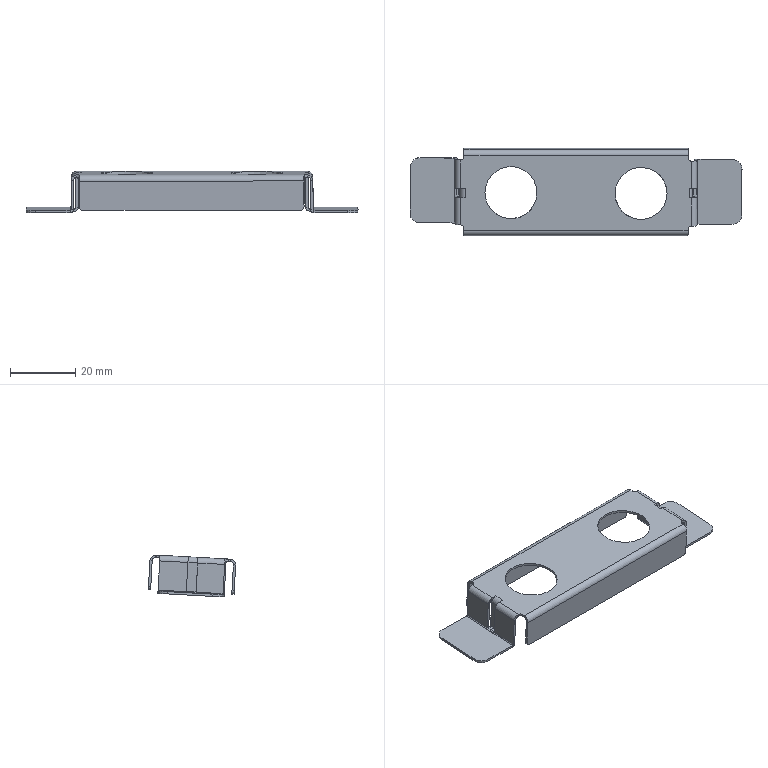Part | STEP file | FNA5401133 | 1 solid | 142 faces | box 102.073 x 26.855 x 12.87 mm | volume 2645 mm3 | spline 70 | cylinder 40 | plane 32 | commonest cylinder face diameters 2 x15 3.4 x8 0.6 x4 6 x4 16 x4 0.4 x2